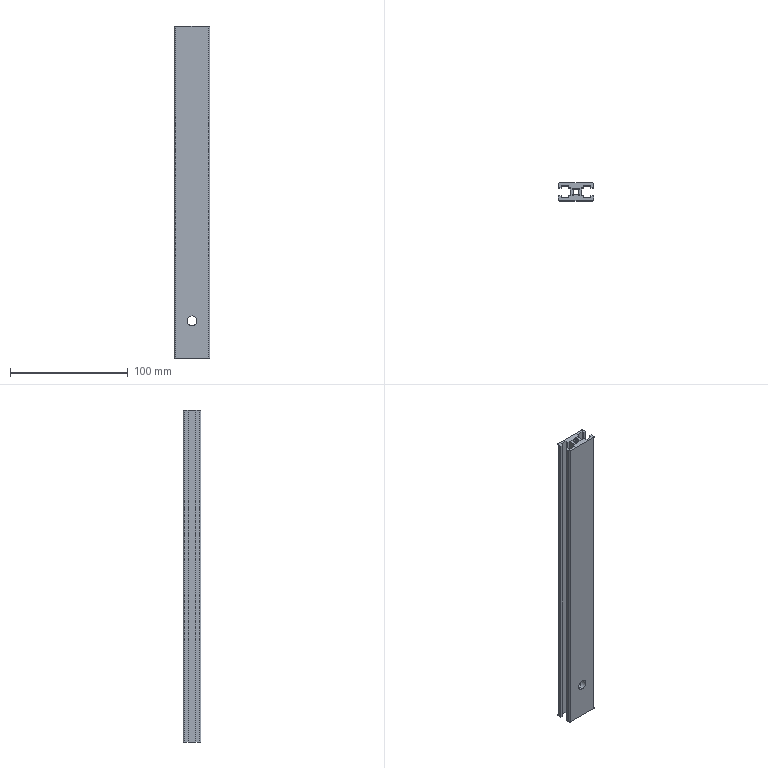Part | NX | features BREP 1 | 1 solid | 74 faces | box 30 x 15 x 282 mm | volume 67355 mm3 | plane 46 | cylinder 28 | commonest cylinder face diameters 1 x12 5 x10 2 x4 8.5 x2